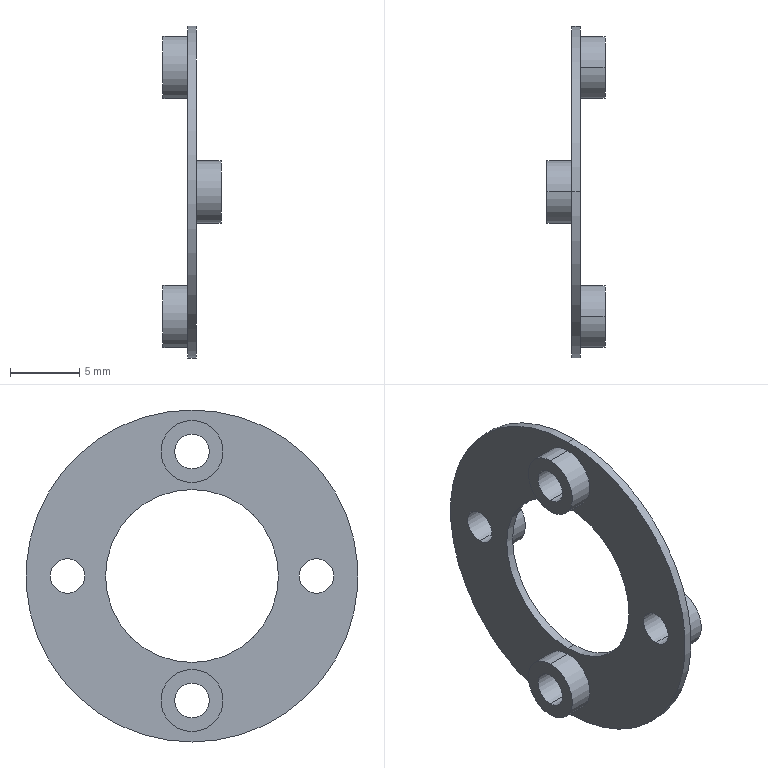Part | STEP file | _DBA11-D25-d10-e12-003.stp | 1 solid | 26 faces | box 4.2 x 24 x 24 mm | volume 265.19 mm3 | cylinder 20 | plane 6 | commonest cylinder face diameters 2.5 x8 4.5 x8 12.5 x2 24 x2
STEP:
#1=CARTESIAN_POINT('',(-1.8,0.,6.75));
#2=VERTEX_POINT('',#1);
#3=CARTESIAN_POINT('',(-1.8,0.,11.25));
#4=VERTEX_POINT('',#3);
#5=CARTESIAN_POINT('',(-1.8,0.,9.));
#6=DIRECTION('',(-1.,0.,0.));
#7=DIRECTION('',(0.,0.,1.));
#8=AXIS2_PLACEMENT_3D('',#5,#6,#7);
#9=CIRCLE('',#8,2.25);
#10=EDGE_CURVE('',#2,#4,#9,.T.);
#11=ORIENTED_EDGE('',*,*,#10,.F.);
#12=CARTESIAN_POINT('',(0.,0.,6.75));
#13=VERTEX_POINT('',#12);
#14=CARTESIAN_POINT('',(-1.8,0.,6.75));
#15=DIRECTION('',(1.,0.,0.));
#16=VECTOR('',#15,1000.);
#17=LINE('',#14,#16);
#18=EDGE_CURVE('',#2,#13,#17,.T.);
#19=ORIENTED_EDGE('',*,*,#18,.T.);
#20=CARTESIAN_POINT('',(0.,0.,11.25));
#21=VERTEX_POINT('',#20);
#22=CARTESIAN_POINT('',(0.,0.,9.));
#23=DIRECTION('',(-1.,0.,0.));
#24=DIRECTION('',(0.,0.,1.));
#25=AXIS2_PLACEMENT_3D('',#22,#23,#24);
#26=CIRCLE('',#25,2.25);
#27=EDGE_CURVE('',#13,#21,#26,.T.);
#28=ORIENTED_EDGE('',*,*,#27,.T.);
#29=CARTESIAN_POINT('',(-1.8,0.,11.25));
#30=DIRECTION('',(1.,0.,0.));
#31=VECTOR('',#30,1000.);
#32=LINE('',#29,#31);
#33=EDGE_CURVE('',#4,#21,#32,.T.);
#34=ORIENTED_EDGE('',*,*,#33,.F.);
#35=EDGE_LOOP('',(#11,#19,#28,#34));
#36=FACE_OUTER_BOUND('',#35,.T.);
#37=CARTESIAN_POINT('',(-1.8,0.,9.));
#38=DIRECTION('',(1.,0.,0.));
#39=DIRECTION('',(0.,0.,1.));
#40=AXIS2_PLACEMENT_3D('',#37,#38,#39);
#41=CYLINDRICAL_SURFACE('',#40,2.25);
#42=ADVANCED_FACE('',(#36),#41,.T.);
#43=CARTESIAN_POINT('',(-1.8,0.,-11.25));
#44=VERTEX_POINT('',#43);
#45=CARTESIAN_POINT('',(-1.8,0.,-6.75));
#46=VERTEX_POINT('',#45);
#47=CARTESIAN_POINT('',(-1.8,0.,-9.));
#48=DIRECTION('',(-1.,0.,0.));
#49=DIRECTION('',(0.,0.,1.));
#50=AXIS2_PLACEMENT_3D('',#47,#48,#49);
#51=CIRCLE('',#50,2.25);
#52=EDGE_CURVE('',#44,#46,#51,.T.);
#53=ORIENTED_EDGE('',*,*,#52,.F.);
#54=CARTESIAN_POINT('',(0.,0.,-11.25));
#55=VERTEX_POINT('',#54);
#56=CARTESIAN_POINT('',(-1.8,0.,-11.25));
#57=DIRECTION('',(1.,0.,0.));
#58=VECTOR('',#57,1000.);
#59=LINE('',#56,#58);
#60=EDGE_CURVE('',#44,#55,#59,.T.);
#61=ORIENTED_EDGE('',*,*,#60,.T.);
#62=CARTESIAN_POINT('',(0.,0.,-6.75));
#63=VERTEX_POINT('',#62);
#64=CARTESIAN_POINT('',(0.,0.,-9.));
#65=DIRECTION('',(-1.,0.,0.));
#66=DIRECTION('',(0.,0.,1.));
#67=AXIS2_PLACEMENT_3D('',#64,#65,#66);
#68=CIRCLE('',#67,2.25);
#69=EDGE_CURVE('',#55,#63,#68,.T.);
#70=ORIENTED_EDGE('',*,*,#69,.T.);
#71=CARTESIAN_POINT('',(-1.8,0.,-6.75));
#72=DIRECTION('',(1.,0.,0.));
#73=VECTOR('',#72,1000.);
#74=LINE('',#71,#73);
#75=EDGE_CURVE('',#46,#63,#74,.T.);
#76=ORIENTED_EDGE('',*,*,#75,.F.);
#77=EDGE_LOOP('',(#53,#61,#70,#76));
#78=FACE_OUTER_BOUND('',#77,.T.);
#79=CARTESIAN_POINT('',(-1.8,0.,-9.));
#80=DIRECTION('',(1.,0.,0.));
#81=DIRECTION('',(0.,0.,1.));
#82=AXIS2_PLACEMENT_3D('',#79,#80,#81);
#83=CYLINDRICAL_SURFACE('',#82,2.25);
#84=ADVANCED_FACE('',(#78),#83,.T.);
#85=CARTESIAN_POINT('',(0.6,-9.,2.25));
#86=VERTEX_POINT('',#85);
#87=CARTESIAN_POINT('',(0.6,-9.,-2.25));
#88=VERTEX_POINT('',#87);
#89=CARTESIAN_POINT('',(0.6,-9.,0.));
#90=DIRECTION('',(1.,0.,0.));
#91=DIRECTION('',(0.,0.,-1.));
#92=AXIS2_PLACEMENT_3D('',#89,#90,#91);
#93=CIRCLE('',#92,2.25);
#94=EDGE_CURVE('',#86,#88,#93,.T.);
#95=ORIENTED_EDGE('',*,*,#94,.T.);
#96=CARTESIAN_POINT('',(2.4,-9.,-2.25));
#97=VERTEX_POINT('',#96);
#98=CARTESIAN_POINT('',(0.6,-9.,-2.25));
#99=DIRECTION('',(1.,0.,0.));
#100=VECTOR('',#99,1000.);
#101=LINE('',#98,#100);
#102=EDGE_CURVE('',#88,#97,#101,.T.);
#103=ORIENTED_EDGE('',*,*,#102,.T.);
#104=CARTESIAN_POINT('',(2.4,-9.,2.25));
#105=VERTEX_POINT('',#104);
#106=CARTESIAN_POINT('',(2.4,-9.,0.));
#107=DIRECTION('',(-1.,0.,0.));
#108=DIRECTION('',(0.,0.,1.));
#109=AXIS2_PLACEMENT_3D('',#106,#107,#108);
#110=CIRCLE('',#109,2.25);
#111=EDGE_CURVE('',#97,#105,#110,.T.);
#112=ORIENTED_EDGE('',*,*,#111,.T.);
#113=CARTESIAN_POINT('',(0.6,-9.,2.25));
#114=DIRECTION('',(1.,0.,0.));
#115=VECTOR('',#114,1000.);
#116=LINE('',#113,#115);
#117=EDGE_CURVE('',#86,#105,#116,.T.);
#118=ORIENTED_EDGE('',*,*,#117,.F.);
#119=EDGE_LOOP('',(#95,#103,#112,#118));
#120=FACE_OUTER_BOUND('',#119,.T.);
#121=CARTESIAN_POINT('',(0.6,-9.,0.));
#122=DIRECTION('',(1.,0.,0.));
#123=DIRECTION('',(0.,0.,1.));
#124=AXIS2_PLACEMENT_3D('',#121,#122,#123);
#125=CYLINDRICAL_SURFACE('',#124,2.25);
#126=ADVANCED_FACE('',(#120),#125,.T.);
#127=CARTESIAN_POINT('',(0.6,9.,2.25));
#128=VERTEX_POINT('',#127);
#129=CARTESIAN_POINT('',(0.6,9.,-2.25));
#130=VERTEX_POINT('',#129);
#131=CARTESIAN_POINT('',(0.6,9.,0.));
#132=DIRECTION('',(1.,0.,0.));
#133=DIRECTION('',(0.,0.,-1.));
#134=AXIS2_PLACEMENT_3D('',#131,#132,#133);
#135=CIRCLE('',#134,2.25);
#136=EDGE_CURVE('',#128,#130,#135,.T.);
#137=ORIENTED_EDGE('',*,*,#136,.T.);
#138=CARTESIAN_POINT('',(2.4,9.,-2.25));
#139=VERTEX_POINT('',#138);
#140=CARTESIAN_POINT('',(0.6,9.,-2.25));
#141=DIRECTION('',(1.,0.,0.));
#142=VECTOR('',#141,1000.);
#143=LINE('',#140,#142);
#144=EDGE_CURVE('',#130,#139,#143,.T.);
#145=ORIENTED_EDGE('',*,*,#144,.T.);
#146=CARTESIAN_POINT('',(2.4,9.,2.25));
#147=VERTEX_POINT('',#146);
#148=CARTESIAN_POINT('',(2.4,9.,0.));
#149=DIRECTION('',(-1.,0.,0.));
#150=DIRECTION('',(0.,0.,1.));
#151=AXIS2_PLACEMENT_3D('',#148,#149,#150);
#152=CIRCLE('',#151,2.25);
#153=EDGE_CURVE('',#139,#147,#152,.T.);
#154=ORIENTED_EDGE('',*,*,#153,.T.);
#155=CARTESIAN_POINT('',(0.6,9.,2.25));
#156=DIRECTION('',(1.,0.,0.));
#157=VECTOR('',#156,1000.);
#158=LINE('',#155,#157);
#159=EDGE_CURVE('',#128,#147,#158,.T.);
#160=ORIENTED_EDGE('',*,*,#159,.F.);
#161=EDGE_LOOP('',(#137,#145,#154,#160));
#162=FACE_OUTER_BOUND('',#161,.T.);
#163=CARTESIAN_POINT('',(0.6,9.,0.));
#164=DIRECTION('',(1.,0.,0.));
#165=DIRECTION('',(0.,0.,1.));
#166=AXIS2_PLACEMENT_3D('',#163,#164,#165);
#167=CYLINDRICAL_SURFACE('',#166,2.25);
#168=ADVANCED_FACE('',(#162),#167,.T.);
#169=CARTESIAN_POINT('',(-1.8,0.,-7.75));
#170=VERTEX_POINT('',#169);
#171=CARTESIAN_POINT('',(-1.8,0.,-10.25));
#172=VERTEX_POINT('',#171);
#173=CARTESIAN_POINT('',(-1.8,0.,-9.));
#174=DIRECTION('',(-1.,0.,0.));
#175=DIRECTION('',(0.,0.,1.));
#176=AXIS2_PLACEMENT_3D('',#173,#174,#175);
#177=CIRCLE('',#176,1.25);
#178=EDGE_CURVE('',#170,#172,#177,.T.);
#179=ORIENTED_EDGE('',*,*,#178,.T.);
#180=CARTESIAN_POINT('',(0.6,0.,-10.25));
#181=VERTEX_POINT('',#180);
#182=CARTESIAN_POINT('',(0.6,0.,-10.25));
#183=DIRECTION('',(1.,0.,0.));
#184=VECTOR('',#183,1000.);
#185=LINE('',#182,#184);
#186=EDGE_CURVE('',#172,#181,#185,.T.);
#187=ORIENTED_EDGE('',*,*,#186,.T.);
#188=CARTESIAN_POINT('',(0.6,0.,-7.75));
#189=VERTEX_POINT('',#188);
#190=CARTESIAN_POINT('',(0.6,0.,-9.));
#191=DIRECTION('',(1.,0.,0.));
#192=DIRECTION('',(0.,0.,-1.));
#193=AXIS2_PLACEMENT_3D('',#190,#191,#192);
#194=CIRCLE('',#193,1.25);
#195=EDGE_CURVE('',#181,#189,#194,.T.);
#196=ORIENTED_EDGE('',*,*,#195,.T.);
#197=CARTESIAN_POINT('',(0.6,0.,-7.75));
#198=DIRECTION('',(1.,0.,0.));
#199=VECTOR('',#198,1000.);
#200=LINE('',#197,#199);
#201=EDGE_CURVE('',#170,#189,#200,.T.);
#202=ORIENTED_EDGE('',*,*,#201,.F.);
#203=EDGE_LOOP('',(#179,#187,#196,#202));
#204=FACE_OUTER_BOUND('',#203,.T.);
#205=CARTESIAN_POINT('',(0.6,0.,-9.));
#206=DIRECTION('',(1.,0.,0.));
#207=DIRECTION('',(0.,0.,1.));
#208=AXIS2_PLACEMENT_3D('',#205,#206,#207);
#209=CYLINDRICAL_SURFACE('',#208,1.25);
#210=ADVANCED_FACE('',(#204),#209,.F.);
#211=CARTESIAN_POINT('',(0.,-9.,1.25));
#212=VERTEX_POINT('',#211);
#213=CARTESIAN_POINT('',(0.,-9.,-1.25));
#214=VERTEX_POINT('',#213);
#215=CARTESIAN_POINT('',(0.,-9.,0.));
#216=DIRECTION('',(-1.,0.,0.));
#217=DIRECTION('',(0.,0.,-1.));
#218=AXIS2_PLACEMENT_3D('',#215,#216,#217);
#219=CIRCLE('',#218,1.25);
#220=EDGE_CURVE('',#212,#214,#219,.T.);
#221=ORIENTED_EDGE('',*,*,#220,.T.);
#222=CARTESIAN_POINT('',(2.4,-9.,-1.25));
#223=VERTEX_POINT('',#222);
#224=CARTESIAN_POINT('',(0.6,-9.,-1.25));
#225=DIRECTION('',(1.,0.,0.));
#226=VECTOR('',#225,1000.);
#227=LINE('',#224,#226);
#228=EDGE_CURVE('',#214,#223,#227,.T.);
#229=ORIENTED_EDGE('',*,*,#228,.T.);
#230=CARTESIAN_POINT('',(2.4,-9.,1.25));
#231=VERTEX_POINT('',#230);
#232=CARTESIAN_POINT('',(2.4,-9.,0.));
#233=DIRECTION('',(-1.,0.,0.));
#234=DIRECTION('',(0.,0.,1.));
#235=AXIS2_PLACEMENT_3D('',#232,#233,#234);
#236=CIRCLE('',#235,1.25);
#237=EDGE_CURVE('',#231,#223,#236,.T.);
#238=ORIENTED_EDGE('',*,*,#237,.F.);
#239=CARTESIAN_POINT('',(0.6,-9.,1.25));
#240=DIRECTION('',(1.,0.,0.));
#241=VECTOR('',#240,1000.);
#242=LINE('',#239,#241);
#243=EDGE_CURVE('',#212,#231,#242,.T.);
#244=ORIENTED_EDGE('',*,*,#243,.F.);
#245=EDGE_LOOP('',(#221,#229,#238,#244));
#246=FACE_OUTER_BOUND('',#245,.T.);
#247=CARTESIAN_POINT('',(0.6,-9.,0.));
#248=DIRECTION('',(1.,0.,0.));
#249=DIRECTION('',(0.,0.,1.));
#250=AXIS2_PLACEMENT_3D('',#247,#248,#249);
#251=CYLINDRICAL_SURFACE('',#250,1.25);
#252=ADVANCED_FACE('',(#246),#251,.F.);
#253=CARTESIAN_POINT('',(-1.8,0.,10.25));
#254=VERTEX_POINT('',#253);
#255=CARTESIAN_POINT('',(-1.8,0.,7.75));
#256=VERTEX_POINT('',#255);
#257=CARTESIAN_POINT('',(-1.8,0.,9.));
#258=DIRECTION('',(-1.,0.,0.));
#259=DIRECTION('',(0.,0.,1.));
#260=AXIS2_PLACEMENT_3D('',#257,#258,#259);
#261=CIRCLE('',#260,1.25);
#262=EDGE_CURVE('',#254,#256,#261,.T.);
#263=ORIENTED_EDGE('',*,*,#262,.T.);
#264=CARTESIAN_POINT('',(0.6,0.,7.75));
#265=VERTEX_POINT('',#264);
#266=CARTESIAN_POINT('',(0.6,0.,7.75));
#267=DIRECTION('',(1.,0.,0.));
#268=VECTOR('',#267,1000.);
#269=LINE('',#266,#268);
#270=EDGE_CURVE('',#256,#265,#269,.T.);
#271=ORIENTED_EDGE('',*,*,#270,.T.);
#272=CARTESIAN_POINT('',(0.6,0.,10.25));
#273=VERTEX_POINT('',#272);
#274=CARTESIAN_POINT('',(0.6,0.,9.));
#275=DIRECTION('',(1.,0.,0.));
#276=DIRECTION('',(0.,0.,-1.));
#277=AXIS2_PLACEMENT_3D('',#274,#275,#276);
#278=CIRCLE('',#277,1.25);
#279=EDGE_CURVE('',#265,#273,#278,.T.);
#280=ORIENTED_EDGE('',*,*,#279,.T.);
#281=CARTESIAN_POINT('',(0.6,0.,10.25));
#282=DIRECTION('',(1.,0.,0.));
#283=VECTOR('',#282,1000.);
#284=LINE('',#281,#283);
#285=EDGE_CURVE('',#254,#273,#284,.T.);
#286=ORIENTED_EDGE('',*,*,#285,.F.);
#287=EDGE_LOOP('',(#263,#271,#280,#286));
#288=FACE_OUTER_BOUND('',#287,.T.);
#289=CARTESIAN_POINT('',(0.6,0.,9.));
#290=DIRECTION('',(1.,0.,0.));
#291=DIRECTION('',(0.,0.,1.));
#292=AXIS2_PLACEMENT_3D('',#289,#290,#291);
#293=CYLINDRICAL_SURFACE('',#292,1.25);
#294=ADVANCED_FACE('',(#288),#293,.F.);
#295=CARTESIAN_POINT('',(0.,9.,1.25));
#296=VERTEX_POINT('',#295);
#297=CARTESIAN_POINT('',(0.,9.,-1.25));
#298=VERTEX_POINT('',#297);
#299=CARTESIAN_POINT('',(0.,9.,0.));
#300=DIRECTION('',(-1.,0.,0.));
#301=DIRECTION('',(0.,0.,-1.));
#302=AXIS2_PLACEMENT_3D('',#299,#300,#301);
#303=CIRCLE('',#302,1.25);
#304=EDGE_CURVE('',#296,#298,#303,.T.);
#305=ORIENTED_EDGE('',*,*,#304,.T.);
#306=CARTESIAN_POINT('',(2.4,9.,-1.25));
#307=VERTEX_POINT('',#306);
#308=CARTESIAN_POINT('',(0.6,9.,-1.25));
#309=DIRECTION('',(1.,0.,0.));
#310=VECTOR('',#309,1000.);
#311=LINE('',#308,#310);
#312=EDGE_CURVE('',#298,#307,#311,.T.);
#313=ORIENTED_EDGE('',*,*,#312,.T.);
#314=CARTESIAN_POINT('',(2.4,9.,1.25));
#315=VERTEX_POINT('',#314);
#316=CARTESIAN_POINT('',(2.4,9.,0.));
#317=DIRECTION('',(-1.,0.,0.));
#318=DIRECTION('',(0.,0.,1.));
#319=AXIS2_PLACEMENT_3D('',#316,#317,#318);
#320=CIRCLE('',#319,1.25);
#321=EDGE_CURVE('',#315,#307,#320,.T.);
#322=ORIENTED_EDGE('',*,*,#321,.F.);
#323=CARTESIAN_POINT('',(0.6,9.,1.25));
#324=DIRECTION('',(1.,0.,0.));
#325=VECTOR('',#324,1000.);
#326=LINE('',#323,#325);
#327=EDGE_CURVE('',#296,#315,#326,.T.);
#328=ORIENTED_EDGE('',*,*,#327,.F.);
#329=EDGE_LOOP('',(#305,#313,#322,#328));
#330=FACE_OUTER_BOUND('',#329,.T.);
#331=CARTESIAN_POINT('',(0.6,9.,0.));
#332=DIRECTION('',(1.,0.,0.));
#333=DIRECTION('',(0.,0.,1.));
#334=AXIS2_PLACEMENT_3D('',#331,#332,#333);
#335=CYLINDRICAL_SURFACE('',#334,1.25);
#336=ADVANCED_FACE('',(#330),#335,.F.);
#337=CARTESIAN_POINT('',(0.,0.,-6.25));
#338=VERTEX_POINT('',#337);
#339=CARTESIAN_POINT('',(0.,0.,6.25));
#340=VERTEX_POINT('',#339);
#341=CARTESIAN_POINT('',(0.,0.,0.));
#342=DIRECTION('',(1.,0.,0.));
#343=DIRECTION('',(0.,0.,-1.));
#344=AXIS2_PLACEMENT_3D('',#341,#342,#343);
#345=CIRCLE('',#344,6.25);
#346=EDGE_CURVE('',#338,#340,#345,.T.);
#347=ORIENTED_EDGE('',*,*,#346,.F.);
#348=CARTESIAN_POINT('',(0.6,0.,-6.25));
#349=VERTEX_POINT('',#348);
#350=CARTESIAN_POINT('',(0.6,0.,-6.25));
#351=DIRECTION('',(1.,0.,0.));
#352=VECTOR('',#351,1000.);
#353=LINE('',#350,#352);
#354=EDGE_CURVE('',#338,#349,#353,.T.);
#355=ORIENTED_EDGE('',*,*,#354,.T.);
#356=CARTESIAN_POINT('',(0.6,0.,6.25));
#357=VERTEX_POINT('',#356);
#358=CARTESIAN_POINT('',(0.6,0.,0.));
#359=DIRECTION('',(1.,0.,0.));
#360=DIRECTION('',(0.,0.,-1.));
#361=AXIS2_PLACEMENT_3D('',#358,#359,#360);
#362=CIRCLE('',#361,6.25);
#363=EDGE_CURVE('',#349,#357,#362,.T.);
#364=ORIENTED_EDGE('',*,*,#363,.T.);
#365=CARTESIAN_POINT('',(0.6,0.,6.25));
#366=DIRECTION('',(1.,0.,0.));
#367=VECTOR('',#366,1000.);
#368=LINE('',#365,#367);
#369=EDGE_CURVE('',#340,#357,#368,.T.);
#370=ORIENTED_EDGE('',*,*,#369,.F.);
#371=EDGE_LOOP('',(#347,#355,#364,#370));
#372=FACE_OUTER_BOUND('',#371,.T.);
#373=CARTESIAN_POINT('',(0.6,0.,0.));
#374=DIRECTION('',(1.,0.,0.));
#375=DIRECTION('',(0.,0.,1.));
#376=AXIS2_PLACEMENT_3D('',#373,#374,#375);
#377=CYLINDRICAL_SURFACE('',#376,6.25);
#378=ADVANCED_FACE('',(#372),#377,.F.);
#379=CARTESIAN_POINT('',(0.,0.,12.));
#380=VERTEX_POINT('',#379);
#381=CARTESIAN_POINT('',(0.,0.,-12.));
#382=VERTEX_POINT('',#381);
#383=CARTESIAN_POINT('',(0.,0.,0.));
#384=DIRECTION('',(1.,0.,0.));
#385=DIRECTION('',(0.,0.,-1.));
#386=AXIS2_PLACEMENT_3D('',#383,#384,#385);
#387=CIRCLE('',#386,12.);
#388=EDGE_CURVE('',#380,#382,#387,.T.);
#389=ORIENTED_EDGE('',*,*,#388,.T.);
#390=CARTESIAN_POINT('',(0.6,0.,-12.));
#391=VERTEX_POINT('',#390);
#392=CARTESIAN_POINT('',(0.6,0.,-12.));
#393=DIRECTION('',(1.,0.,0.));
#394=VECTOR('',#393,1000.);
#395=LINE('',#392,#394);
#396=EDGE_CURVE('',#382,#391,#395,.T.);
#397=ORIENTED_EDGE('',*,*,#396,.T.);
#398=CARTESIAN_POINT('',(0.6,0.,12.));
#399=VERTEX_POINT('',#398);
#400=CARTESIAN_POINT('',(0.6,0.,0.));
#401=DIRECTION('',(1.,0.,0.));
#402=DIRECTION('',(0.,0.,-1.));
#403=AXIS2_PLACEMENT_3D('',#400,#401,#402);
#404=CIRCLE('',#403,12.);
#405=EDGE_CURVE('',#399,#391,#404,.T.);
#406=ORIENTED_EDGE('',*,*,#405,.F.);
#407=CARTESIAN_POINT('',(0.6,0.,12.));
#408=DIRECTION('',(1.,0.,0.));
#409=VECTOR('',#408,1000.);
#410=LINE('',#407,#409);
#411=EDGE_CURVE('',#380,#399,#410,.T.);
#412=ORIENTED_EDGE('',*,*,#411,.F.);
#413=EDGE_LOOP('',(#389,#397,#406,#412));
#414=FACE_OUTER_BOUND('',#413,.T.);
#415=CARTESIAN_POINT('',(0.6,0.,0.));
#416=DIRECTION('',(1.,0.,0.));
#417=DIRECTION('',(0.,0.,1.));
#418=AXIS2_PLACEMENT_3D('',#415,#416,#417);
#419=CYLINDRICAL_SURFACE('',#418,12.);
#420=ADVANCED_FACE('',(#414),#419,.T.);
#421=ORIENTED_EDGE('',*,*,#388,.F.);
#422=CARTESIAN_POINT('',(0.,0.,0.));
#423=DIRECTION('',(1.,0.,0.));
#424=DIRECTION('',(0.,0.,-1.));
#425=AXIS2_PLACEMENT_3D('',#422,#423,#424);
#426=CIRCLE('',#425,12.);
#427=EDGE_CURVE('',#382,#380,#426,.T.);
#428=ORIENTED_EDGE('',*,*,#427,.F.);
#429=EDGE_LOOP('',(#421,#428));
#430=FACE_OUTER_BOUND('',#429,.T.);
#431=CARTESIAN_POINT('',(0.,0.,9.));
#432=DIRECTION('',(-1.,0.,0.));
#433=DIRECTION('',(0.,0.,1.));
#434=AXIS2_PLACEMENT_3D('',#431,#432,#433);
#435=CIRCLE('',#434,2.25);
#436=EDGE_CURVE('',#21,#13,#435,.T.);
#437=ORIENTED_EDGE('',*,*,#436,.F.);
#438=ORIENTED_EDGE('',*,*,#27,.F.);
#439=EDGE_LOOP('',(#437,#438));
#440=FACE_BOUND('',#439,.T.);
#441=CARTESIAN_POINT('',(0.,0.,-9.));
#442=DIRECTION('',(-1.,0.,0.));
#443=DIRECTION('',(0.,0.,1.));
#444=AXIS2_PLACEMENT_3D('',#441,#442,#443);
#445=CIRCLE('',#444,2.25);
#446=EDGE_CURVE('',#63,#55,#445,.T.);
#447=ORIENTED_EDGE('',*,*,#446,.F.);
#448=ORIENTED_EDGE('',*,*,#69,.F.);
#449=EDGE_LOOP('',(#447,#448));
#450=FACE_BOUND('',#449,.T.);
#451=ORIENTED_EDGE('',*,*,#220,.F.);
#452=CARTESIAN_POINT('',(0.,-9.,0.));
#453=DIRECTION('',(-1.,0.,0.));
#454=DIRECTION('',(0.,0.,-1.));
#455=AXIS2_PLACEMENT_3D('',#452,#453,#454);
#456=CIRCLE('',#455,1.25);
#457=EDGE_CURVE('',#214,#212,#456,.T.);
#458=ORIENTED_EDGE('',*,*,#457,.F.);
#459=EDGE_LOOP('',(#451,#458));
#460=FACE_BOUND('',#459,.T.);
#461=ORIENTED_EDGE('',*,*,#304,.F.);
#462=CARTESIAN_POINT('',(0.,9.,0.));
#463=DIRECTION('',(-1.,0.,0.));
#464=DIRECTION('',(0.,0.,-1.));
#465=AXIS2_PLACEMENT_3D('',#462,#463,#464);
#466=CIRCLE('',#465,1.25);
#467=EDGE_CURVE('',#298,#296,#466,.T.);
#468=ORIENTED_EDGE('',*,*,#467,.F.);
#469=EDGE_LOOP('',(#461,#468));
#470=FACE_BOUND('',#469,.T.);
#471=CARTESIAN_POINT('',(0.,0.,0.));
#472=DIRECTION('',(1.,0.,0.));
#473=DIRECTION('',(0.,0.,-1.));
#474=AXIS2_PLACEMENT_3D('',#471,#472,#473);
#475=CIRCLE('',#474,6.25);
#476=EDGE_CURVE('',#340,#338,#475,.T.);
#477=ORIENTED_EDGE('',*,*,#476,.T.);
#478=ORIENTED_EDGE('',*,*,#346,.T.);
#479=EDGE_LOOP('',(#477,#478));
#480=FACE_BOUND('',#479,.T.);
#481=CARTESIAN_POINT('',(0.,0.,0.));
#482=DIRECTION('',(1.,0.,0.));
#483=DIRECTION('',(0.,1.,0.));
#484=AXIS2_PLACEMENT_3D('',#481,#482,#483);
#485=PLANE('',#484);
#486=ADVANCED_FACE('',(#430,#440,#450,#460,#470,#480),#485,.F.);
#487=ORIENTED_EDGE('',*,*,#396,.F.);
#488=ORIENTED_EDGE('',*,*,#427,.T.);
#489=ORIENTED_EDGE('',*,*,#411,.T.);
#490=CARTESIAN_POINT('',(0.6,0.,0.));
#491=DIRECTION('',(1.,0.,0.));
#492=DIRECTION('',(0.,0.,-1.));
#493=AXIS2_PLACEMENT_3D('',#490,#491,#492);
#494=CIRCLE('',#493,12.);
#495=EDGE_CURVE('',#391,#399,#494,.T.);
#496=ORIENTED_EDGE('',*,*,#495,.F.);
#497=EDGE_LOOP('',(#487,#488,#489,#496));
#498=FACE_OUTER_BOUND('',#497,.T.);
#499=CARTESIAN_POINT('',(0.6,0.,0.));
#500=DIRECTION('',(1.,0.,0.));
#501=DIRECTION('',(0.,0.,1.));
#502=AXIS2_PLACEMENT_3D('',#499,#500,#501);
#503=CYLINDRICAL_SURFACE('',#502,12.);
#504=ADVANCED_FACE('',(#498),#503,.T.);
#505=ORIENTED_EDGE('',*,*,#405,.T.);
#506=ORIENTED_EDGE('',*,*,#495,.T.);
#507=EDGE_LOOP('',(#505,#506));
#508=FACE_OUTER_BOUND('',#507,.T.);
#509=ORIENTED_EDGE('',*,*,#94,.F.);
#510=CARTESIAN_POINT('',(0.6,-9.,0.));
#511=DIRECTION('',(1.,0.,0.));
#512=DIRECTION('',(0.,0.,-1.));
#513=AXIS2_PLACEMENT_3D('',#510,#511,#512);
#514=CIRCLE('',#513,2.25);
#515=EDGE_CURVE('',#88,#86,#514,.T.);
#516=ORIENTED_EDGE('',*,*,#515,.F.);
#517=EDGE_LOOP('',(#509,#516));
#518=FACE_BOUND('',#517,.T.);
#519=ORIENTED_EDGE('',*,*,#136,.F.);
#520=CARTESIAN_POINT('',(0.6,9.,0.));
#521=DIRECTION('',(1.,0.,0.));
#522=DIRECTION('',(0.,0.,-1.));
#523=AXIS2_PLACEMENT_3D('',#520,#521,#522);
#524=CIRCLE('',#523,2.25);
#525=EDGE_CURVE('',#130,#128,#524,.T.);
#526=ORIENTED_EDGE('',*,*,#525,.F.);
#527=EDGE_LOOP('',(#519,#526));
#528=FACE_BOUND('',#527,.T.);
#529=CARTESIAN_POINT('',(0.6,0.,-9.));
#530=DIRECTION('',(1.,0.,0.));
#531=DIRECTION('',(0.,0.,-1.));
#532=AXIS2_PLACEMENT_3D('',#529,#530,#531);
#533=CIRCLE('',#532,1.25);
#534=EDGE_CURVE('',#189,#181,#533,.T.);
#535=ORIENTED_EDGE('',*,*,#534,.F.);
#536=ORIENTED_EDGE('',*,*,#195,.F.);
#537=EDGE_LOOP('',(#535,#536));
#538=FACE_BOUND('',#537,.T.);
#539=CARTESIAN_POINT('',(0.6,0.,9.));
#540=DIRECTION('',(1.,0.,0.));
#541=DIRECTION('',(0.,0.,-1.));
#542=AXIS2_PLACEMENT_3D('',#539,#540,#541);
#543=CIRCLE('',#542,1.25);
#544=EDGE_CURVE('',#273,#265,#543,.T.);
#545=ORIENTED_EDGE('',*,*,#544,.F.);
#546=ORIENTED_EDGE('',*,*,#279,.F.);
#547=EDGE_LOOP('',(#545,#546));
#548=FACE_BOUND('',#547,.T.);
#549=CARTESIAN_POINT('',(0.6,0.,0.));
#550=DIRECTION('',(1.,0.,0.));
#551=DIRECTION('',(0.,0.,-1.));
#552=AXIS2_PLACEMENT_3D('',#549,#550,#551);
#553=CIRCLE('',#552,6.25);
#554=EDGE_CURVE('',#357,#349,#553,.T.);
#555=ORIENTED_EDGE('',*,*,#554,.F.);
#556=ORIENTED_EDGE('',*,*,#363,.F.);
#557=EDGE_LOOP('',(#555,#556));
#558=FACE_BOUND('',#557,.T.);
#559=CARTESIAN_POINT('',(0.6,0.,0.));
#560=DIRECTION('',(1.,0.,0.));
#561=DIRECTION('',(0.,1.,0.));
#562=AXIS2_PLACEMENT_3D('',#559,#560,#561);
#563=PLANE('',#562);
#564=ADVANCED_FACE('',(#508,#518,#528,#538,#548,#558),#563,.T.);
#565=ORIENTED_EDGE('',*,*,#354,.F.);
#566=ORIENTED_EDGE('',*,*,#476,.F.);
#567=ORIENTED_EDGE('',*,*,#369,.T.);
#568=ORIENTED_EDGE('',*,*,#554,.T.);
#569=EDGE_LOOP('',(#565,#566,#567,#568));
#570=FACE_OUTER_BOUND('',#569,.T.);
#571=CARTESIAN_POINT('',(0.6,0.,0.));
#572=DIRECTION('',(1.,0.,0.));
#573=DIRECTION('',(0.,0.,1.));
#574=AXIS2_PLACEMENT_3D('',#571,#572,#573);
#575=CYLINDRICAL_SURFACE('',#574,6.25);
#576=ADVANCED_FACE('',(#570),#575,.F.);
#577=ORIENTED_EDGE('',*,*,#312,.F.);
#578=ORIENTED_EDGE('',*,*,#467,.T.);
#579=ORIENTED_EDGE('',*,*,#327,.T.);
#580=CARTESIAN_POINT('',(2.4,9.,0.));
#581=DIRECTION('',(-1.,0.,0.));
#582=DIRECTION('',(0.,0.,1.));
#583=AXIS2_PLACEMENT_3D('',#580,#581,#582);
#584=CIRCLE('',#583,1.25);
#585=EDGE_CURVE('',#307,#315,#584,.T.);
#586=ORIENTED_EDGE('',*,*,#585,.F.);
#587=EDGE_LOOP('',(#577,#578,#579,#586));
#588=FACE_OUTER_BOUND('',#587,.T.);
#589=CARTESIAN_POINT('',(0.6,9.,0.));
#590=DIRECTION('',(1.,0.,0.));
#591=DIRECTION('',(0.,0.,1.));
#592=AXIS2_PLACEMENT_3D('',#589,#590,#591);
#593=CYLINDRICAL_SURFACE('',#592,1.25);
#594=ADVANCED_FACE('',(#588),#593,.F.);
#595=ORIENTED_EDGE('',*,*,#270,.F.);
#596=CARTESIAN_POINT('',(-1.8,0.,9.));
#597=DIRECTION('',(-1.,0.,0.));
#598=DIRECTION('',(0.,0.,1.));
#599=AXIS2_PLACEMENT_3D('',#596,#597,#598);
#600=CIRCLE('',#599,1.25);
#601=EDGE_CURVE('',#256,#254,#600,.T.);
#602=ORIENTED_EDGE('',*,*,#601,.T.);
#603=ORIENTED_EDGE('',*,*,#285,.T.);
#604=ORIENTED_EDGE('',*,*,#544,.T.);
#605=EDGE_LOOP('',(#595,#602,#603,#604));
#606=FACE_OUTER_BOUND('',#605,.T.);
#607=CARTESIAN_POINT('',(0.6,0.,9.));
#608=DIRECTION('',(1.,0.,0.));
#609=DIRECTION('',(0.,0.,1.));
#610=AXIS2_PLACEMENT_3D('',#607,#608,#609);
#611=CYLINDRICAL_SURFACE('',#610,1.25);
#612=ADVANCED_FACE('',(#606),#611,.F.);
#613=ORIENTED_EDGE('',*,*,#228,.F.);
#614=ORIENTED_EDGE('',*,*,#457,.T.);
#615=ORIENTED_EDGE('',*,*,#243,.T.);
#616=CARTESIAN_POINT('',(2.4,-9.,0.));
#617=DIRECTION('',(-1.,0.,0.));
#618=DIRECTION('',(0.,0.,1.));
#619=AXIS2_PLACEMENT_3D('',#616,#617,#618);
#620=CIRCLE('',#619,1.25);
#621=EDGE_CURVE('',#223,#231,#620,.T.);
#622=ORIENTED_EDGE('',*,*,#621,.F.);
#623=EDGE_LOOP('',(#613,#614,#615,#622));
#624=FACE_OUTER_BOUND('',#623,.T.);
#625=CARTESIAN_POINT('',(0.6,-9.,0.));
#626=DIRECTION('',(1.,0.,0.));
#627=DIRECTION('',(0.,0.,1.));
#628=AXIS2_PLACEMENT_3D('',#625,#626,#627);
#629=CYLINDRICAL_SURFACE('',#628,1.25);
#630=ADVANCED_FACE('',(#624),#629,.F.);
#631=ORIENTED_EDGE('',*,*,#186,.F.);
#632=CARTESIAN_POINT('',(-1.8,0.,-9.));
#633=DIRECTION('',(-1.,0.,0.));
#634=DIRECTION('',(0.,0.,1.));
#635=AXIS2_PLACEMENT_3D('',#632,#633,#634);
#636=CIRCLE('',#635,1.25);
#637=EDGE_CURVE('',#172,#170,#636,.T.);
#638=ORIENTED_EDGE('',*,*,#637,.T.);
#639=ORIENTED_EDGE('',*,*,#201,.T.);
#640=ORIENTED_EDGE('',*,*,#534,.T.);
#641=EDGE_LOOP('',(#631,#638,#639,#640));
#642=FACE_OUTER_BOUND('',#641,.T.);
#643=CARTESIAN_POINT('',(0.6,0.,-9.));
#644=DIRECTION('',(1.,0.,0.));
#645=DIRECTION('',(0.,0.,1.));
#646=AXIS2_PLACEMENT_3D('',#643,#644,#645);
#647=CYLINDRICAL_SURFACE('',#646,1.25);
#648=ADVANCED_FACE('',(#642),#647,.F.);
#649=ORIENTED_EDGE('',*,*,#144,.F.);
#650=ORIENTED_EDGE('',*,*,#525,.T.);
#651=ORIENTED_EDGE('',*,*,#159,.T.);
#652=CARTESIAN_POINT('',(2.4,9.,0.));
#653=DIRECTION('',(-1.,0.,0.));
#654=DIRECTION('',(0.,0.,1.));
#655=AXIS2_PLACEMENT_3D('',#652,#653,#654);
#656=CIRCLE('',#655,2.25);
#657=EDGE_CURVE('',#147,#139,#656,.T.);
#658=ORIENTED_EDGE('',*,*,#657,.T.);
#659=EDGE_LOOP('',(#649,#650,#651,#658));
#660=FACE_OUTER_BOUND('',#659,.T.);
#661=CARTESIAN_POINT('',(0.6,9.,0.));
#662=DIRECTION('',(1.,0.,0.));
#663=DIRECTION('',(0.,0.,1.));
#664=AXIS2_PLACEMENT_3D('',#661,#662,#663);
#665=CYLINDRICAL_SURFACE('',#664,2.25);
#666=ADVANCED_FACE('',(#660),#665,.T.);
#667=ORIENTED_EDGE('',*,*,#657,.F.);
#668=ORIENTED_EDGE('',*,*,#153,.F.);
#669=EDGE_LOOP('',(#667,#668));
#670=FACE_OUTER_BOUND('',#669,.T.);
#671=ORIENTED_EDGE('',*,*,#321,.T.);
#672=ORIENTED_EDGE('',*,*,#585,.T.);
#673=EDGE_LOOP('',(#671,#672));
#674=FACE_BOUND('',#673,.T.);
#675=CARTESIAN_POINT('',(2.4,6.75,0.));
#676=DIRECTION('',(1.,0.,0.));
#677=DIRECTION('',(0.,1.,0.));
#678=AXIS2_PLACEMENT_3D('',#675,#676,#677);
#679=PLANE('',#678);
#680=ADVANCED_FACE('',(#670,#674),#679,.T.);
#681=ORIENTED_EDGE('',*,*,#102,.F.);
#682=ORIENTED_EDGE('',*,*,#515,.T.);
#683=ORIENTED_EDGE('',*,*,#117,.T.);
#684=CARTESIAN_POINT('',(2.4,-9.,0.));
#685=DIRECTION('',(-1.,0.,0.));
#686=DIRECTION('',(0.,0.,1.));
#687=AXIS2_PLACEMENT_3D('',#684,#685,#686);
#688=CIRCLE('',#687,2.25);
#689=EDGE_CURVE('',#105,#97,#688,.T.);
#690=ORIENTED_EDGE('',*,*,#689,.T.);
#691=EDGE_LOOP('',(#681,#682,#683,#690));
#692=FACE_OUTER_BOUND('',#691,.T.);
#693=CARTESIAN_POINT('',(0.6,-9.,0.));
#694=DIRECTION('',(1.,0.,0.));
#695=DIRECTION('',(0.,0.,1.));
#696=AXIS2_PLACEMENT_3D('',#693,#694,#695);
#697=CYLINDRICAL_SURFACE('',#696,2.25);
#698=ADVANCED_FACE('',(#692),#697,.T.);
#699=ORIENTED_EDGE('',*,*,#689,.F.);
#700=ORIENTED_EDGE('',*,*,#111,.F.);
#701=EDGE_LOOP('',(#699,#700));
#702=FACE_OUTER_BOUND('',#701,.T.);
#703=ORIENTED_EDGE('',*,*,#237,.T.);
#704=ORIENTED_EDGE('',*,*,#621,.T.);
#705=EDGE_LOOP('',(#703,#704));
#706=FACE_BOUND('',#705,.T.);
#707=CARTESIAN_POINT('',(2.4,-11.25,0.));
#708=DIRECTION('',(1.,0.,0.));
#709=DIRECTION('',(0.,1.,0.));
#710=AXIS2_PLACEMENT_3D('',#707,#708,#709);
#711=PLANE('',#710);
#712=ADVANCED_FACE('',(#702,#706),#711,.T.);
#713=CARTESIAN_POINT('',(-1.8,0.,-9.));
#714=DIRECTION('',(-1.,0.,0.));
#715=DIRECTION('',(0.,0.,1.));
#716=AXIS2_PLACEMENT_3D('',#713,#714,#715);
#717=CIRCLE('',#716,2.25);
#718=EDGE_CURVE('',#46,#44,#717,.T.);
#719=ORIENTED_EDGE('',*,*,#718,.T.);
#720=ORIENTED_EDGE('',*,*,#52,.T.);
#721=EDGE_LOOP('',(#719,#720));
#722=FACE_OUTER_BOUND('',#721,.T.);
#723=ORIENTED_EDGE('',*,*,#178,.F.);
#724=ORIENTED_EDGE('',*,*,#637,.F.);
#725=EDGE_LOOP('',(#723,#724));
#726=FACE_BOUND('',#725,.T.);
#727=CARTESIAN_POINT('',(-1.8,0.,-7.75));
#728=DIRECTION('',(-1.,0.,0.));
#729=DIRECTION('',(0.,0.,1.));
#730=AXIS2_PLACEMENT_3D('',#727,#728,#729);
#731=PLANE('',#730);
#732=ADVANCED_FACE('',(#722,#726),#731,.T.);
#733=ORIENTED_EDGE('',*,*,#60,.F.);
#734=ORIENTED_EDGE('',*,*,#718,.F.);
#735=ORIENTED_EDGE('',*,*,#75,.T.);
#736=ORIENTED_EDGE('',*,*,#446,.T.);
#737=EDGE_LOOP('',(#733,#734,#735,#736));
#738=FACE_OUTER_BOUND('',#737,.T.);
#739=CARTESIAN_POINT('',(-1.8,0.,-9.));
#740=DIRECTION('',(1.,0.,0.));
#741=DIRECTION('',(0.,0.,1.));
#742=AXIS2_PLACEMENT_3D('',#739,#740,#741);
#743=CYLINDRICAL_SURFACE('',#742,2.25);
#744=ADVANCED_FACE('',(#738),#743,.T.);
#745=CARTESIAN_POINT('',(-1.8,0.,9.));
#746=DIRECTION('',(-1.,0.,0.));
#747=DIRECTION('',(0.,0.,1.));
#748=AXIS2_PLACEMENT_3D('',#745,#746,#747);
#749=CIRCLE('',#748,2.25);
#750=EDGE_CURVE('',#4,#2,#749,.T.);
#751=ORIENTED_EDGE('',*,*,#750,.T.);
#752=ORIENTED_EDGE('',*,*,#10,.T.);
#753=EDGE_LOOP('',(#751,#752));
#754=FACE_OUTER_BOUND('',#753,.T.);
#755=ORIENTED_EDGE('',*,*,#262,.F.);
#756=ORIENTED_EDGE('',*,*,#601,.F.);
#757=EDGE_LOOP('',(#755,#756));
#758=FACE_BOUND('',#757,.T.);
#759=CARTESIAN_POINT('',(-1.8,0.,10.25));
#760=DIRECTION('',(-1.,0.,0.));
#761=DIRECTION('',(0.,0.,1.));
#762=AXIS2_PLACEMENT_3D('',#759,#760,#761);
#763=PLANE('',#762);
#764=ADVANCED_FACE('',(#754,#758),#763,.T.);
#765=ORIENTED_EDGE('',*,*,#18,.F.);
#766=ORIENTED_EDGE('',*,*,#750,.F.);
#767=ORIENTED_EDGE('',*,*,#33,.T.);
#768=ORIENTED_EDGE('',*,*,#436,.T.);
#769=EDGE_LOOP('',(#765,#766,#767,#768));
#770=FACE_OUTER_BOUND('',#769,.T.);
#771=CARTESIAN_POINT('',(-1.8,0.,9.));
#772=DIRECTION('',(1.,0.,0.));
#773=DIRECTION('',(0.,0.,1.));
#774=AXIS2_PLACEMENT_3D('',#771,#772,#773);
#775=CYLINDRICAL_SURFACE('',#774,2.25);
#776=ADVANCED_FACE('',(#770),#775,.T.);
#777=CLOSED_SHELL('',(#42,#84,#126,#168,#210,#252,#294,#336,#378,#420,#486,#504,#564,#576,#594,#612,#630,#648,#666,#680,#698,#712,#732,#744,#764,#776));
#778=MANIFOLD_SOLID_BREP('',#777);
#779=CARTESIAN_POINT('',(0.,0.,0.));
#780=DIRECTION('',(0.,0.,1.));
#781=DIRECTION('',(1.,0.,0.));
#782=AXIS2_PLACEMENT_3D('',#779,#780,#781);
#783=(LENGTH_UNIT()NAMED_UNIT(*)SI_UNIT(.MILLI.,.METRE.));
#784=UNCERTAINTY_MEASURE_WITH_UNIT(LENGTH_MEASURE(0.00001),#783,'','');
#785=(NAMED_UNIT(*)PLANE_ANGLE_UNIT()SI_UNIT($,.RADIAN.));
#786=(NAMED_UNIT(*)SI_UNIT($,.STERADIAN.)SOLID_ANGLE_UNIT());
#787=(GEOMETRIC_REPRESENTATION_CONTEXT(3)GLOBAL_UNCERTAINTY_ASSIGNED_CONTEXT((#784))GLOBAL_UNIT_ASSIGNED_CONTEXT((#783,#785,#786))REPRESENTATION_CONTEXT('',''));
#788=ADVANCED_BREP_SHAPE_REPRESENTATION('',(#778,#782),#787);